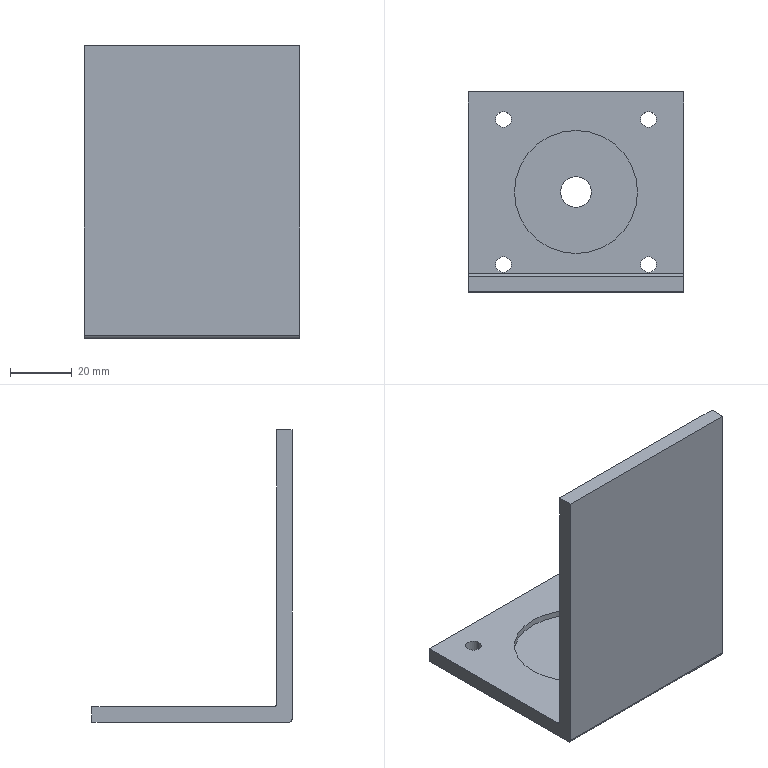Part | SolidWorks | features ICE 4, Fillet 2, Extrusion 1 | 1 solid | 23 faces | box 70 x 65 x 95 mm | volume 51093 mm3 | cylinder 14 | plane 9 | commonest cylinder face diameters 5.1 x8 2 x2 10 x2 40 x2
STEP:
#1=CARTESIAN_POINT('',(-5.,0.,0.));
#2=VERTEX_POINT('',#1);
#3=CARTESIAN_POINT('',(5.,0.,0.));
#4=VERTEX_POINT('',#3);
#5=CARTESIAN_POINT('',(0.,0.,0.));
#6=DIRECTION('',(0.,0.,1.));
#7=DIRECTION('',(1.,0.,0.));
#8=AXIS2_PLACEMENT_3D('',#5,#6,#7);
#9=CIRCLE('',#8,5.);
#10=EDGE_CURVE('',#2,#4,#9,.T.);
#11=ORIENTED_EDGE('',*,*,#10,.F.);
#12=CARTESIAN_POINT('',(-5.,0.,3.));
#13=VERTEX_POINT('',#12);
#14=CARTESIAN_POINT('',(-5.,0.,0.));
#15=DIRECTION('',(0.,0.,1.));
#16=VECTOR('',#15,1000.);
#17=LINE('',#14,#16);
#18=EDGE_CURVE('',#2,#13,#17,.T.);
#19=ORIENTED_EDGE('',*,*,#18,.T.);
#20=CARTESIAN_POINT('',(5.,0.,3.));
#21=VERTEX_POINT('',#20);
#22=CARTESIAN_POINT('',(0.,0.,3.));
#23=DIRECTION('',(0.,0.,1.));
#24=DIRECTION('',(1.,0.,0.));
#25=AXIS2_PLACEMENT_3D('',#22,#23,#24);
#26=CIRCLE('',#25,5.);
#27=EDGE_CURVE('',#13,#21,#26,.T.);
#28=ORIENTED_EDGE('',*,*,#27,.T.);
#29=CARTESIAN_POINT('',(5.,0.,0.));
#30=DIRECTION('',(0.,0.,1.));
#31=VECTOR('',#30,1000.);
#32=LINE('',#29,#31);
#33=EDGE_CURVE('',#4,#21,#32,.T.);
#34=ORIENTED_EDGE('',*,*,#33,.F.);
#35=EDGE_LOOP('',(#11,#19,#28,#34));
#36=FACE_OUTER_BOUND('',#35,.T.);
#37=CARTESIAN_POINT('',(0.,0.,0.));
#38=DIRECTION('',(0.,0.,1.));
#39=DIRECTION('',(1.,0.,0.));
#40=AXIS2_PLACEMENT_3D('',#37,#38,#39);
#41=CYLINDRICAL_SURFACE('',#40,5.);
#42=ADVANCED_FACE('',(#36),#41,.F.);
#43=CARTESIAN_POINT('',(-20.,0.,3.));
#44=VERTEX_POINT('',#43);
#45=CARTESIAN_POINT('',(20.,0.,3.));
#46=VERTEX_POINT('',#45);
#47=CARTESIAN_POINT('',(0.,0.,3.));
#48=DIRECTION('',(0.,0.,1.));
#49=DIRECTION('',(1.,0.,0.));
#50=AXIS2_PLACEMENT_3D('',#47,#48,#49);
#51=CIRCLE('',#50,20.);
#52=EDGE_CURVE('',#44,#46,#51,.T.);
#53=ORIENTED_EDGE('',*,*,#52,.F.);
#54=CARTESIAN_POINT('',(-20.,0.,5.));
#55=VERTEX_POINT('',#54);
#56=CARTESIAN_POINT('',(-20.,0.,3.));
#57=DIRECTION('',(0.,0.,1.));
#58=VECTOR('',#57,1000.);
#59=LINE('',#56,#58);
#60=EDGE_CURVE('',#44,#55,#59,.T.);
#61=ORIENTED_EDGE('',*,*,#60,.T.);
#62=CARTESIAN_POINT('',(20.,0.,5.));
#63=VERTEX_POINT('',#62);
#64=CARTESIAN_POINT('',(0.,0.,5.));
#65=DIRECTION('',(0.,0.,1.));
#66=DIRECTION('',(1.,0.,0.));
#67=AXIS2_PLACEMENT_3D('',#64,#65,#66);
#68=CIRCLE('',#67,20.);
#69=EDGE_CURVE('',#55,#63,#68,.T.);
#70=ORIENTED_EDGE('',*,*,#69,.T.);
#71=CARTESIAN_POINT('',(20.,0.,3.));
#72=DIRECTION('',(0.,0.,1.));
#73=VECTOR('',#72,1000.);
#74=LINE('',#71,#73);
#75=EDGE_CURVE('',#46,#63,#74,.T.);
#76=ORIENTED_EDGE('',*,*,#75,.F.);
#77=EDGE_LOOP('',(#53,#61,#70,#76));
#78=FACE_OUTER_BOUND('',#77,.T.);
#79=CARTESIAN_POINT('',(0.,0.,3.));
#80=DIRECTION('',(0.,0.,1.));
#81=DIRECTION('',(1.,0.,0.));
#82=AXIS2_PLACEMENT_3D('',#79,#80,#81);
#83=CYLINDRICAL_SURFACE('',#82,20.);
#84=ADVANCED_FACE('',(#78),#83,.F.);
#85=CARTESIAN_POINT('',(-26.12,-23.57,0.));
#86=VERTEX_POINT('',#85);
#87=CARTESIAN_POINT('',(-21.02,-23.57,0.));
#88=VERTEX_POINT('',#87);
#89=CARTESIAN_POINT('',(-23.57,-23.57,0.));
#90=DIRECTION('',(0.,0.,1.));
#91=DIRECTION('',(1.,0.,0.));
#92=AXIS2_PLACEMENT_3D('',#89,#90,#91);
#93=CIRCLE('',#92,2.55);
#94=EDGE_CURVE('',#86,#88,#93,.T.);
#95=ORIENTED_EDGE('',*,*,#94,.F.);
#96=CARTESIAN_POINT('',(-26.12,-23.57,5.));
#97=VERTEX_POINT('',#96);
#98=CARTESIAN_POINT('',(-26.12,-23.57,0.));
#99=DIRECTION('',(0.,0.,1.));
#100=VECTOR('',#99,1000.);
#101=LINE('',#98,#100);
#102=EDGE_CURVE('',#86,#97,#101,.T.);
#103=ORIENTED_EDGE('',*,*,#102,.T.);
#104=CARTESIAN_POINT('',(-21.02,-23.57,5.));
#105=VERTEX_POINT('',#104);
#106=CARTESIAN_POINT('',(-23.57,-23.57,5.));
#107=DIRECTION('',(0.,0.,1.));
#108=DIRECTION('',(1.,0.,0.));
#109=AXIS2_PLACEMENT_3D('',#106,#107,#108);
#110=CIRCLE('',#109,2.55);
#111=EDGE_CURVE('',#97,#105,#110,.T.);
#112=ORIENTED_EDGE('',*,*,#111,.T.);
#113=CARTESIAN_POINT('',(-21.02,-23.57,0.));
#114=DIRECTION('',(0.,0.,1.));
#115=VECTOR('',#114,1000.);
#116=LINE('',#113,#115);
#117=EDGE_CURVE('',#88,#105,#116,.T.);
#118=ORIENTED_EDGE('',*,*,#117,.F.);
#119=EDGE_LOOP('',(#95,#103,#112,#118));
#120=FACE_OUTER_BOUND('',#119,.T.);
#121=CARTESIAN_POINT('',(-23.57,-23.57,0.));
#122=DIRECTION('',(0.,0.,1.));
#123=DIRECTION('',(1.,0.,0.));
#124=AXIS2_PLACEMENT_3D('',#121,#122,#123);
#125=CYLINDRICAL_SURFACE('',#124,2.55);
#126=ADVANCED_FACE('',(#120),#125,.F.);
#127=CARTESIAN_POINT('',(21.02,-23.57,0.));
#128=VERTEX_POINT('',#127);
#129=CARTESIAN_POINT('',(26.12,-23.57,0.));
#130=VERTEX_POINT('',#129);
#131=CARTESIAN_POINT('',(23.57,-23.57,0.));
#132=DIRECTION('',(0.,0.,1.));
#133=DIRECTION('',(1.,0.,0.));
#134=AXIS2_PLACEMENT_3D('',#131,#132,#133);
#135=CIRCLE('',#134,2.55);
#136=EDGE_CURVE('',#128,#130,#135,.T.);
#137=ORIENTED_EDGE('',*,*,#136,.F.);
#138=CARTESIAN_POINT('',(21.02,-23.57,5.));
#139=VERTEX_POINT('',#138);
#140=CARTESIAN_POINT('',(21.02,-23.57,0.));
#141=DIRECTION('',(0.,0.,1.));
#142=VECTOR('',#141,1000.);
#143=LINE('',#140,#142);
#144=EDGE_CURVE('',#128,#139,#143,.T.);
#145=ORIENTED_EDGE('',*,*,#144,.T.);
#146=CARTESIAN_POINT('',(26.12,-23.57,5.));
#147=VERTEX_POINT('',#146);
#148=CARTESIAN_POINT('',(23.57,-23.57,5.));
#149=DIRECTION('',(0.,0.,1.));
#150=DIRECTION('',(1.,0.,0.));
#151=AXIS2_PLACEMENT_3D('',#148,#149,#150);
#152=CIRCLE('',#151,2.55);
#153=EDGE_CURVE('',#139,#147,#152,.T.);
#154=ORIENTED_EDGE('',*,*,#153,.T.);
#155=CARTESIAN_POINT('',(26.12,-23.57,0.));
#156=DIRECTION('',(0.,0.,1.));
#157=VECTOR('',#156,1000.);
#158=LINE('',#155,#157);
#159=EDGE_CURVE('',#130,#147,#158,.T.);
#160=ORIENTED_EDGE('',*,*,#159,.F.);
#161=EDGE_LOOP('',(#137,#145,#154,#160));
#162=FACE_OUTER_BOUND('',#161,.T.);
#163=CARTESIAN_POINT('',(23.57,-23.57,0.));
#164=DIRECTION('',(0.,0.,1.));
#165=DIRECTION('',(1.,0.,0.));
#166=AXIS2_PLACEMENT_3D('',#163,#164,#165);
#167=CYLINDRICAL_SURFACE('',#166,2.55);
#168=ADVANCED_FACE('',(#162),#167,.F.);
#169=CARTESIAN_POINT('',(21.02,23.57,0.));
#170=VERTEX_POINT('',#169);
#171=CARTESIAN_POINT('',(26.12,23.57,0.));
#172=VERTEX_POINT('',#171);
#173=CARTESIAN_POINT('',(23.57,23.57,0.));
#174=DIRECTION('',(0.,0.,1.));
#175=DIRECTION('',(1.,0.,0.));
#176=AXIS2_PLACEMENT_3D('',#173,#174,#175);
#177=CIRCLE('',#176,2.55);
#178=EDGE_CURVE('',#170,#172,#177,.T.);
#179=ORIENTED_EDGE('',*,*,#178,.F.);
#180=CARTESIAN_POINT('',(21.02,23.57,5.));
#181=VERTEX_POINT('',#180);
#182=CARTESIAN_POINT('',(21.02,23.57,0.));
#183=DIRECTION('',(0.,0.,1.));
#184=VECTOR('',#183,1000.);
#185=LINE('',#182,#184);
#186=EDGE_CURVE('',#170,#181,#185,.T.);
#187=ORIENTED_EDGE('',*,*,#186,.T.);
#188=CARTESIAN_POINT('',(26.12,23.57,5.));
#189=VERTEX_POINT('',#188);
#190=CARTESIAN_POINT('',(23.57,23.57,5.));
#191=DIRECTION('',(0.,0.,1.));
#192=DIRECTION('',(1.,0.,0.));
#193=AXIS2_PLACEMENT_3D('',#190,#191,#192);
#194=CIRCLE('',#193,2.55);
#195=EDGE_CURVE('',#181,#189,#194,.T.);
#196=ORIENTED_EDGE('',*,*,#195,.T.);
#197=CARTESIAN_POINT('',(26.12,23.57,0.));
#198=DIRECTION('',(0.,0.,1.));
#199=VECTOR('',#198,1000.);
#200=LINE('',#197,#199);
#201=EDGE_CURVE('',#172,#189,#200,.T.);
#202=ORIENTED_EDGE('',*,*,#201,.F.);
#203=EDGE_LOOP('',(#179,#187,#196,#202));
#204=FACE_OUTER_BOUND('',#203,.T.);
#205=CARTESIAN_POINT('',(23.57,23.57,0.));
#206=DIRECTION('',(0.,0.,1.));
#207=DIRECTION('',(1.,0.,0.));
#208=AXIS2_PLACEMENT_3D('',#205,#206,#207);
#209=CYLINDRICAL_SURFACE('',#208,2.55);
#210=ADVANCED_FACE('',(#204),#209,.F.);
#211=CARTESIAN_POINT('',(-26.12,23.57,0.));
#212=VERTEX_POINT('',#211);
#213=CARTESIAN_POINT('',(-21.02,23.57,0.));
#214=VERTEX_POINT('',#213);
#215=CARTESIAN_POINT('',(-23.57,23.57,0.));
#216=DIRECTION('',(0.,0.,1.));
#217=DIRECTION('',(1.,0.,0.));
#218=AXIS2_PLACEMENT_3D('',#215,#216,#217);
#219=CIRCLE('',#218,2.55);
#220=EDGE_CURVE('',#212,#214,#219,.T.);
#221=ORIENTED_EDGE('',*,*,#220,.F.);
#222=CARTESIAN_POINT('',(-26.12,23.57,5.));
#223=VERTEX_POINT('',#222);
#224=CARTESIAN_POINT('',(-26.12,23.57,0.));
#225=DIRECTION('',(0.,0.,1.));
#226=VECTOR('',#225,1000.);
#227=LINE('',#224,#226);
#228=EDGE_CURVE('',#212,#223,#227,.T.);
#229=ORIENTED_EDGE('',*,*,#228,.T.);
#230=CARTESIAN_POINT('',(-21.02,23.57,5.));
#231=VERTEX_POINT('',#230);
#232=CARTESIAN_POINT('',(-23.57,23.57,5.));
#233=DIRECTION('',(0.,0.,1.));
#234=DIRECTION('',(1.,0.,0.));
#235=AXIS2_PLACEMENT_3D('',#232,#233,#234);
#236=CIRCLE('',#235,2.55);
#237=EDGE_CURVE('',#223,#231,#236,.T.);
#238=ORIENTED_EDGE('',*,*,#237,.T.);
#239=CARTESIAN_POINT('',(-21.02,23.57,0.));
#240=DIRECTION('',(0.,0.,1.));
#241=VECTOR('',#240,1000.);
#242=LINE('',#239,#241);
#243=EDGE_CURVE('',#214,#231,#242,.T.);
#244=ORIENTED_EDGE('',*,*,#243,.F.);
#245=EDGE_LOOP('',(#221,#229,#238,#244));
#246=FACE_OUTER_BOUND('',#245,.T.);
#247=CARTESIAN_POINT('',(-23.57,23.57,0.));
#248=DIRECTION('',(0.,0.,1.));
#249=DIRECTION('',(1.,0.,0.));
#250=AXIS2_PLACEMENT_3D('',#247,#248,#249);
#251=CYLINDRICAL_SURFACE('',#250,2.55);
#252=ADVANCED_FACE('',(#246),#251,.F.);
#253=CARTESIAN_POINT('',(-35.,32.5,0.));
#254=VERTEX_POINT('',#253);
#255=CARTESIAN_POINT('',(35.,32.5,0.));
#256=VERTEX_POINT('',#255);
#257=CARTESIAN_POINT('',(-35.,32.5,0.));
#258=DIRECTION('',(1.,0.,0.));
#259=VECTOR('',#258,1000.);
#260=LINE('',#257,#259);
#261=EDGE_CURVE('',#254,#256,#260,.T.);
#262=ORIENTED_EDGE('',*,*,#261,.F.);
#263=CARTESIAN_POINT('',(-35.,32.5,5.));
#264=VERTEX_POINT('',#263);
#265=CARTESIAN_POINT('',(-35.,32.5,5.));
#266=DIRECTION('',(0.,0.,-1.));
#267=VECTOR('',#266,1000.);
#268=LINE('',#265,#267);
#269=EDGE_CURVE('',#264,#254,#268,.T.);
#270=ORIENTED_EDGE('',*,*,#269,.F.);
#271=CARTESIAN_POINT('',(35.,32.5,5.));
#272=VERTEX_POINT('',#271);
#273=CARTESIAN_POINT('',(-35.,32.5,5.));
#274=DIRECTION('',(1.,0.,0.));
#275=VECTOR('',#274,1000.);
#276=LINE('',#273,#275);
#277=EDGE_CURVE('',#264,#272,#276,.T.);
#278=ORIENTED_EDGE('',*,*,#277,.T.);
#279=CARTESIAN_POINT('',(35.,32.5,5.));
#280=DIRECTION('',(0.,0.,-1.));
#281=VECTOR('',#280,1000.);
#282=LINE('',#279,#281);
#283=EDGE_CURVE('',#272,#256,#282,.T.);
#284=ORIENTED_EDGE('',*,*,#283,.T.);
#285=EDGE_LOOP('',(#262,#270,#278,#284));
#286=FACE_OUTER_BOUND('',#285,.T.);
#287=CARTESIAN_POINT('',(-35.,32.5,5.));
#288=DIRECTION('',(0.,1.,0.));
#289=DIRECTION('',(0.,0.,1.));
#290=AXIS2_PLACEMENT_3D('',#287,#288,#289);
#291=PLANE('',#290);
#292=ADVANCED_FACE('',(#286),#291,.T.);
#293=CARTESIAN_POINT('',(-35.,-31.5,0.));
#294=VERTEX_POINT('',#293);
#295=CARTESIAN_POINT('',(-35.,-32.5,0.));
#296=DIRECTION('',(0.,1.,0.));
#297=VECTOR('',#296,1000.);
#298=LINE('',#295,#297);
#299=EDGE_CURVE('',#294,#254,#298,.T.);
#300=ORIENTED_EDGE('',*,*,#299,.F.);
#301=CARTESIAN_POINT('',(-35.,-32.5,1.));
#302=VERTEX_POINT('',#301);
#303=CARTESIAN_POINT('',(-35.,-31.5,1.));
#304=DIRECTION('',(-1.,0.,0.));
#305=DIRECTION('',(0.,0.,1.));
#306=AXIS2_PLACEMENT_3D('',#303,#304,#305);
#307=CIRCLE('',#306,1.);
#308=EDGE_CURVE('',#294,#302,#307,.T.);
#309=ORIENTED_EDGE('',*,*,#308,.T.);
#310=CARTESIAN_POINT('',(-35.,-32.5,95.));
#311=VERTEX_POINT('',#310);
#312=CARTESIAN_POINT('',(-35.,-32.5,5.));
#313=DIRECTION('',(0.,0.,-1.));
#314=VECTOR('',#313,1000.);
#315=LINE('',#312,#314);
#316=EDGE_CURVE('',#311,#302,#315,.T.);
#317=ORIENTED_EDGE('',*,*,#316,.F.);
#318=CARTESIAN_POINT('',(-35.,-27.5,95.));
#319=VERTEX_POINT('',#318);
#320=CARTESIAN_POINT('',(-35.,-32.5,95.));
#321=DIRECTION('',(0.,-1.,0.));
#322=VECTOR('',#321,1000.);
#323=LINE('',#320,#322);
#324=EDGE_CURVE('',#319,#311,#323,.T.);
#325=ORIENTED_EDGE('',*,*,#324,.F.);
#326=CARTESIAN_POINT('',(-35.,-27.5,6.));
#327=VERTEX_POINT('',#326);
#328=CARTESIAN_POINT('',(-35.,-27.5,95.));
#329=DIRECTION('',(0.,0.,-1.));
#330=VECTOR('',#329,1000.);
#331=LINE('',#328,#330);
#332=EDGE_CURVE('',#319,#327,#331,.T.);
#333=ORIENTED_EDGE('',*,*,#332,.T.);
#334=CARTESIAN_POINT('',(-35.,-26.5,5.));
#335=VERTEX_POINT('',#334);
#336=CARTESIAN_POINT('',(-35.,-26.5,6.));
#337=DIRECTION('',(1.,0.,0.));
#338=DIRECTION('',(0.,0.,1.));
#339=AXIS2_PLACEMENT_3D('',#336,#337,#338);
#340=CIRCLE('',#339,1.);
#341=EDGE_CURVE('',#327,#335,#340,.T.);
#342=ORIENTED_EDGE('',*,*,#341,.T.);
#343=CARTESIAN_POINT('',(-35.,-32.5,5.));
#344=DIRECTION('',(0.,1.,0.));
#345=VECTOR('',#344,1000.);
#346=LINE('',#343,#345);
#347=EDGE_CURVE('',#335,#264,#346,.T.);
#348=ORIENTED_EDGE('',*,*,#347,.T.);
#349=ORIENTED_EDGE('',*,*,#269,.T.);
#350=EDGE_LOOP('',(#300,#309,#317,#325,#333,#342,#348,#349));
#351=FACE_OUTER_BOUND('',#350,.T.);
#352=CARTESIAN_POINT('',(-35.,-32.5,5.));
#353=DIRECTION('',(-1.,0.,0.));
#354=DIRECTION('',(0.,0.,1.));
#355=AXIS2_PLACEMENT_3D('',#352,#353,#354);
#356=PLANE('',#355);
#357=ADVANCED_FACE('',(#351),#356,.T.);
#358=ORIENTED_EDGE('',*,*,#316,.T.);
#359=CARTESIAN_POINT('',(35.,-32.5,1.));
#360=VERTEX_POINT('',#359);
#361=CARTESIAN_POINT('',(-35.,-32.5,1.));
#362=DIRECTION('',(1.,0.,0.));
#363=VECTOR('',#362,1000.);
#364=LINE('',#361,#363);
#365=EDGE_CURVE('',#302,#360,#364,.T.);
#366=ORIENTED_EDGE('',*,*,#365,.T.);
#367=CARTESIAN_POINT('',(35.,-32.5,95.));
#368=VERTEX_POINT('',#367);
#369=CARTESIAN_POINT('',(35.,-32.5,5.));
#370=DIRECTION('',(0.,0.,-1.));
#371=VECTOR('',#370,1000.);
#372=LINE('',#369,#371);
#373=EDGE_CURVE('',#368,#360,#372,.T.);
#374=ORIENTED_EDGE('',*,*,#373,.F.);
#375=CARTESIAN_POINT('',(-35.,-32.5,95.));
#376=DIRECTION('',(1.,0.,0.));
#377=VECTOR('',#376,1000.);
#378=LINE('',#375,#377);
#379=EDGE_CURVE('',#311,#368,#378,.T.);
#380=ORIENTED_EDGE('',*,*,#379,.F.);
#381=EDGE_LOOP('',(#358,#366,#374,#380));
#382=FACE_OUTER_BOUND('',#381,.T.);
#383=CARTESIAN_POINT('',(-35.,-32.5,5.));
#384=DIRECTION('',(0.,1.,0.));
#385=DIRECTION('',(0.,0.,1.));
#386=AXIS2_PLACEMENT_3D('',#383,#384,#385);
#387=PLANE('',#386);
#388=ADVANCED_FACE('',(#382),#387,.F.);
#389=ORIENTED_EDGE('',*,*,#373,.T.);
#390=CARTESIAN_POINT('',(35.,-31.5,0.));
#391=VERTEX_POINT('',#390);
#392=CARTESIAN_POINT('',(35.,-31.5,1.));
#393=DIRECTION('',(1.,0.,0.));
#394=DIRECTION('',(0.,0.,1.));
#395=AXIS2_PLACEMENT_3D('',#392,#393,#394);
#396=CIRCLE('',#395,1.);
#397=EDGE_CURVE('',#360,#391,#396,.T.);
#398=ORIENTED_EDGE('',*,*,#397,.T.);
#399=CARTESIAN_POINT('',(35.,-32.5,0.));
#400=DIRECTION('',(0.,1.,0.));
#401=VECTOR('',#400,1000.);
#402=LINE('',#399,#401);
#403=EDGE_CURVE('',#391,#256,#402,.T.);
#404=ORIENTED_EDGE('',*,*,#403,.T.);
#405=ORIENTED_EDGE('',*,*,#283,.F.);
#406=CARTESIAN_POINT('',(35.,-26.5,5.));
#407=VERTEX_POINT('',#406);
#408=CARTESIAN_POINT('',(35.,-32.5,5.));
#409=DIRECTION('',(0.,1.,0.));
#410=VECTOR('',#409,1000.);
#411=LINE('',#408,#410);
#412=EDGE_CURVE('',#407,#272,#411,.T.);
#413=ORIENTED_EDGE('',*,*,#412,.F.);
#414=CARTESIAN_POINT('',(35.,-27.5,6.));
#415=VERTEX_POINT('',#414);
#416=CARTESIAN_POINT('',(35.,-26.5,6.));
#417=DIRECTION('',(-1.,0.,0.));
#418=DIRECTION('',(0.,0.,1.));
#419=AXIS2_PLACEMENT_3D('',#416,#417,#418);
#420=CIRCLE('',#419,1.);
#421=EDGE_CURVE('',#407,#415,#420,.T.);
#422=ORIENTED_EDGE('',*,*,#421,.T.);
#423=CARTESIAN_POINT('',(35.,-27.5,95.));
#424=VERTEX_POINT('',#423);
#425=CARTESIAN_POINT('',(35.,-27.5,95.));
#426=DIRECTION('',(0.,0.,-1.));
#427=VECTOR('',#426,1000.);
#428=LINE('',#425,#427);
#429=EDGE_CURVE('',#424,#415,#428,.T.);
#430=ORIENTED_EDGE('',*,*,#429,.F.);
#431=CARTESIAN_POINT('',(35.,-32.5,95.));
#432=DIRECTION('',(0.,1.,0.));
#433=VECTOR('',#432,1000.);
#434=LINE('',#431,#433);
#435=EDGE_CURVE('',#368,#424,#434,.T.);
#436=ORIENTED_EDGE('',*,*,#435,.F.);
#437=EDGE_LOOP('',(#389,#398,#404,#405,#413,#422,#430,#436));
#438=FACE_OUTER_BOUND('',#437,.T.);
#439=CARTESIAN_POINT('',(35.,-32.5,5.));
#440=DIRECTION('',(-1.,0.,0.));
#441=DIRECTION('',(0.,0.,1.));
#442=AXIS2_PLACEMENT_3D('',#439,#440,#441);
#443=PLANE('',#442);
#444=ADVANCED_FACE('',(#438),#443,.F.);
#445=CARTESIAN_POINT('',(0.,0.,5.));
#446=DIRECTION('',(0.,0.,1.));
#447=DIRECTION('',(1.,0.,0.));
#448=AXIS2_PLACEMENT_3D('',#445,#446,#447);
#449=CIRCLE('',#448,20.);
#450=EDGE_CURVE('',#63,#55,#449,.T.);
#451=ORIENTED_EDGE('',*,*,#450,.F.);
#452=ORIENTED_EDGE('',*,*,#69,.F.);
#453=EDGE_LOOP('',(#451,#452));
#454=FACE_BOUND('',#453,.T.);
#455=ORIENTED_EDGE('',*,*,#347,.F.);
#456=CARTESIAN_POINT('',(0.,-26.5,5.));
#457=DIRECTION('',(1.,0.,0.));
#458=VECTOR('',#457,1000.);
#459=LINE('',#456,#458);
#460=EDGE_CURVE('',#335,#407,#459,.T.);
#461=ORIENTED_EDGE('',*,*,#460,.T.);
#462=ORIENTED_EDGE('',*,*,#412,.T.);
#463=ORIENTED_EDGE('',*,*,#277,.F.);
#464=EDGE_LOOP('',(#455,#461,#462,#463));
#465=FACE_OUTER_BOUND('',#464,.T.);
#466=CARTESIAN_POINT('',(-23.57,-23.57,5.));
#467=DIRECTION('',(0.,0.,1.));
#468=DIRECTION('',(1.,0.,0.));
#469=AXIS2_PLACEMENT_3D('',#466,#467,#468);
#470=CIRCLE('',#469,2.55);
#471=EDGE_CURVE('',#105,#97,#470,.T.);
#472=ORIENTED_EDGE('',*,*,#471,.F.);
#473=ORIENTED_EDGE('',*,*,#111,.F.);
#474=EDGE_LOOP('',(#472,#473));
#475=FACE_BOUND('',#474,.T.);
#476=CARTESIAN_POINT('',(23.57,-23.57,5.));
#477=DIRECTION('',(0.,0.,1.));
#478=DIRECTION('',(1.,0.,0.));
#479=AXIS2_PLACEMENT_3D('',#476,#477,#478);
#480=CIRCLE('',#479,2.55);
#481=EDGE_CURVE('',#147,#139,#480,.T.);
#482=ORIENTED_EDGE('',*,*,#481,.F.);
#483=ORIENTED_EDGE('',*,*,#153,.F.);
#484=EDGE_LOOP('',(#482,#483));
#485=FACE_BOUND('',#484,.T.);
#486=CARTESIAN_POINT('',(23.57,23.57,5.));
#487=DIRECTION('',(0.,0.,1.));
#488=DIRECTION('',(1.,0.,0.));
#489=AXIS2_PLACEMENT_3D('',#486,#487,#488);
#490=CIRCLE('',#489,2.55);
#491=EDGE_CURVE('',#189,#181,#490,.T.);
#492=ORIENTED_EDGE('',*,*,#491,.F.);
#493=ORIENTED_EDGE('',*,*,#195,.F.);
#494=EDGE_LOOP('',(#492,#493));
#495=FACE_BOUND('',#494,.T.);
#496=CARTESIAN_POINT('',(-23.57,23.57,5.));
#497=DIRECTION('',(0.,0.,1.));
#498=DIRECTION('',(1.,0.,0.));
#499=AXIS2_PLACEMENT_3D('',#496,#497,#498);
#500=CIRCLE('',#499,2.55);
#501=EDGE_CURVE('',#231,#223,#500,.T.);
#502=ORIENTED_EDGE('',*,*,#501,.F.);
#503=ORIENTED_EDGE('',*,*,#237,.F.);
#504=EDGE_LOOP('',(#502,#503));
#505=FACE_BOUND('',#504,.T.);
#506=CARTESIAN_POINT('',(0.,0.,5.));
#507=DIRECTION('',(0.,0.,1.));
#508=DIRECTION('',(1.,0.,0.));
#509=AXIS2_PLACEMENT_3D('',#506,#507,#508);
#510=PLANE('',#509);
#511=ADVANCED_FACE('',(#454,#465,#475,#485,#495,#505),#510,.T.);
#512=CARTESIAN_POINT('',(0.,0.,0.));
#513=DIRECTION('',(0.,0.,1.));
#514=DIRECTION('',(1.,0.,0.));
#515=AXIS2_PLACEMENT_3D('',#512,#513,#514);
#516=CIRCLE('',#515,5.);
#517=EDGE_CURVE('',#4,#2,#516,.T.);
#518=ORIENTED_EDGE('',*,*,#517,.T.);
#519=ORIENTED_EDGE('',*,*,#10,.T.);
#520=EDGE_LOOP('',(#518,#519));
#521=FACE_BOUND('',#520,.T.);
#522=CARTESIAN_POINT('',(-23.57,-23.57,0.));
#523=DIRECTION('',(0.,0.,1.));
#524=DIRECTION('',(1.,0.,0.));
#525=AXIS2_PLACEMENT_3D('',#522,#523,#524);
#526=CIRCLE('',#525,2.55);
#527=EDGE_CURVE('',#88,#86,#526,.T.);
#528=ORIENTED_EDGE('',*,*,#527,.T.);
#529=ORIENTED_EDGE('',*,*,#94,.T.);
#530=EDGE_LOOP('',(#528,#529));
#531=FACE_BOUND('',#530,.T.);
#532=CARTESIAN_POINT('',(23.57,-23.57,0.));
#533=DIRECTION('',(0.,0.,1.));
#534=DIRECTION('',(1.,0.,0.));
#535=AXIS2_PLACEMENT_3D('',#532,#533,#534);
#536=CIRCLE('',#535,2.55);
#537=EDGE_CURVE('',#130,#128,#536,.T.);
#538=ORIENTED_EDGE('',*,*,#537,.T.);
#539=ORIENTED_EDGE('',*,*,#136,.T.);
#540=EDGE_LOOP('',(#538,#539));
#541=FACE_BOUND('',#540,.T.);
#542=CARTESIAN_POINT('',(23.57,23.57,0.));
#543=DIRECTION('',(0.,0.,1.));
#544=DIRECTION('',(1.,0.,0.));
#545=AXIS2_PLACEMENT_3D('',#542,#543,#544);
#546=CIRCLE('',#545,2.55);
#547=EDGE_CURVE('',#172,#170,#546,.T.);
#548=ORIENTED_EDGE('',*,*,#547,.T.);
#549=ORIENTED_EDGE('',*,*,#178,.T.);
#550=EDGE_LOOP('',(#548,#549));
#551=FACE_BOUND('',#550,.T.);
#552=CARTESIAN_POINT('',(-23.57,23.57,0.));
#553=DIRECTION('',(0.,0.,1.));
#554=DIRECTION('',(1.,0.,0.));
#555=AXIS2_PLACEMENT_3D('',#552,#553,#554);
#556=CIRCLE('',#555,2.55);
#557=EDGE_CURVE('',#214,#212,#556,.T.);
#558=ORIENTED_EDGE('',*,*,#557,.T.);
#559=ORIENTED_EDGE('',*,*,#220,.T.);
#560=EDGE_LOOP('',(#558,#559));
#561=FACE_BOUND('',#560,.T.);
#562=ORIENTED_EDGE('',*,*,#403,.F.);
#563=CARTESIAN_POINT('',(0.,-31.5,0.));
#564=DIRECTION('',(-1.,0.,0.));
#565=VECTOR('',#564,1000.);
#566=LINE('',#563,#565);
#567=EDGE_CURVE('',#391,#294,#566,.T.);
#568=ORIENTED_EDGE('',*,*,#567,.T.);
#569=ORIENTED_EDGE('',*,*,#299,.T.);
#570=ORIENTED_EDGE('',*,*,#261,.T.);
#571=EDGE_LOOP('',(#562,#568,#569,#570));
#572=FACE_OUTER_BOUND('',#571,.T.);
#573=CARTESIAN_POINT('',(0.,0.,0.));
#574=DIRECTION('',(0.,0.,1.));
#575=DIRECTION('',(1.,0.,0.));
#576=AXIS2_PLACEMENT_3D('',#573,#574,#575);
#577=PLANE('',#576);
#578=ADVANCED_FACE('',(#521,#531,#541,#551,#561,#572),#577,.F.);
#579=ORIENTED_EDGE('',*,*,#228,.F.);
#580=ORIENTED_EDGE('',*,*,#557,.F.);
#581=ORIENTED_EDGE('',*,*,#243,.T.);
#582=ORIENTED_EDGE('',*,*,#501,.T.);
#583=EDGE_LOOP('',(#579,#580,#581,#582));
#584=FACE_OUTER_BOUND('',#583,.T.);
#585=CARTESIAN_POINT('',(-23.57,23.57,0.));
#586=DIRECTION('',(0.,0.,1.));
#587=DIRECTION('',(1.,0.,0.));
#588=AXIS2_PLACEMENT_3D('',#585,#586,#587);
#589=CYLINDRICAL_SURFACE('',#588,2.55);
#590=ADVANCED_FACE('',(#584),#589,.F.);
#591=ORIENTED_EDGE('',*,*,#186,.F.);
#592=ORIENTED_EDGE('',*,*,#547,.F.);
#593=ORIENTED_EDGE('',*,*,#201,.T.);
#594=ORIENTED_EDGE('',*,*,#491,.T.);
#595=EDGE_LOOP('',(#591,#592,#593,#594));
#596=FACE_OUTER_BOUND('',#595,.T.);
#597=CARTESIAN_POINT('',(23.57,23.57,0.));
#598=DIRECTION('',(0.,0.,1.));
#599=DIRECTION('',(1.,0.,0.));
#600=AXIS2_PLACEMENT_3D('',#597,#598,#599);
#601=CYLINDRICAL_SURFACE('',#600,2.55);
#602=ADVANCED_FACE('',(#596),#601,.F.);
#603=ORIENTED_EDGE('',*,*,#144,.F.);
#604=ORIENTED_EDGE('',*,*,#537,.F.);
#605=ORIENTED_EDGE('',*,*,#159,.T.);
#606=ORIENTED_EDGE('',*,*,#481,.T.);
#607=EDGE_LOOP('',(#603,#604,#605,#606));
#608=FACE_OUTER_BOUND('',#607,.T.);
#609=CARTESIAN_POINT('',(23.57,-23.57,0.));
#610=DIRECTION('',(0.,0.,1.));
#611=DIRECTION('',(1.,0.,0.));
#612=AXIS2_PLACEMENT_3D('',#609,#610,#611);
#613=CYLINDRICAL_SURFACE('',#612,2.55);
#614=ADVANCED_FACE('',(#608),#613,.F.);
#615=ORIENTED_EDGE('',*,*,#102,.F.);
#616=ORIENTED_EDGE('',*,*,#527,.F.);
#617=ORIENTED_EDGE('',*,*,#117,.T.);
#618=ORIENTED_EDGE('',*,*,#471,.T.);
#619=EDGE_LOOP('',(#615,#616,#617,#618));
#620=FACE_OUTER_BOUND('',#619,.T.);
#621=CARTESIAN_POINT('',(-23.57,-23.57,0.));
#622=DIRECTION('',(0.,0.,1.));
#623=DIRECTION('',(1.,0.,0.));
#624=AXIS2_PLACEMENT_3D('',#621,#622,#623);
#625=CYLINDRICAL_SURFACE('',#624,2.55);
#626=ADVANCED_FACE('',(#620),#625,.F.);
#627=ORIENTED_EDGE('',*,*,#429,.T.);
#628=CARTESIAN_POINT('',(-35.,-27.5,6.));
#629=DIRECTION('',(-1.,0.,0.));
#630=VECTOR('',#629,1000.);
#631=LINE('',#628,#630);
#632=EDGE_CURVE('',#415,#327,#631,.T.);
#633=ORIENTED_EDGE('',*,*,#632,.T.);
#634=ORIENTED_EDGE('',*,*,#332,.F.);
#635=CARTESIAN_POINT('',(-35.,-27.5,95.));
#636=DIRECTION('',(-1.,0.,0.));
#637=VECTOR('',#636,1000.);
#638=LINE('',#635,#637);
#639=EDGE_CURVE('',#424,#319,#638,.T.);
#640=ORIENTED_EDGE('',*,*,#639,.F.);
#641=EDGE_LOOP('',(#627,#633,#634,#640));
#642=FACE_OUTER_BOUND('',#641,.T.);
#643=CARTESIAN_POINT('',(-35.,-27.5,95.));
#644=DIRECTION('',(0.,-1.,0.));
#645=DIRECTION('',(0.,0.,-1.));
#646=AXIS2_PLACEMENT_3D('',#643,#644,#645);
#647=PLANE('',#646);
#648=ADVANCED_FACE('',(#642),#647,.F.);
#649=ORIENTED_EDGE('',*,*,#324,.T.);
#650=ORIENTED_EDGE('',*,*,#379,.T.);
#651=ORIENTED_EDGE('',*,*,#435,.T.);
#652=ORIENTED_EDGE('',*,*,#639,.T.);
#653=EDGE_LOOP('',(#649,#650,#651,#652));
#654=FACE_OUTER_BOUND('',#653,.T.);
#655=CARTESIAN_POINT('',(0.,0.,95.));
#656=DIRECTION('',(0.,0.,-1.));
#657=DIRECTION('',(-1.,0.,0.));
#658=AXIS2_PLACEMENT_3D('',#655,#656,#657);
#659=PLANE('',#658);
#660=ADVANCED_FACE('',(#654),#659,.F.);
#661=ORIENTED_EDGE('',*,*,#421,.F.);
#662=ORIENTED_EDGE('',*,*,#460,.F.);
#663=ORIENTED_EDGE('',*,*,#341,.F.);
#664=ORIENTED_EDGE('',*,*,#632,.F.);
#665=EDGE_LOOP('',(#661,#662,#663,#664));
#666=FACE_OUTER_BOUND('',#665,.T.);
#667=CARTESIAN_POINT('',(-35.,-26.5,6.));
#668=DIRECTION('',(-1.,0.,0.));
#669=DIRECTION('',(0.,0.,1.));
#670=AXIS2_PLACEMENT_3D('',#667,#668,#669);
#671=CYLINDRICAL_SURFACE('',#670,1.);
#672=ADVANCED_FACE('',(#666),#671,.F.);
#673=ORIENTED_EDGE('',*,*,#308,.F.);
#674=ORIENTED_EDGE('',*,*,#567,.F.);
#675=ORIENTED_EDGE('',*,*,#397,.F.);
#676=ORIENTED_EDGE('',*,*,#365,.F.);
#677=EDGE_LOOP('',(#673,#674,#675,#676));
#678=FACE_OUTER_BOUND('',#677,.T.);
#679=CARTESIAN_POINT('',(-35.,-31.5,1.));
#680=DIRECTION('',(1.,0.,0.));
#681=DIRECTION('',(0.,0.,-1.));
#682=AXIS2_PLACEMENT_3D('',#679,#680,#681);
#683=CYLINDRICAL_SURFACE('',#682,1.);
#684=ADVANCED_FACE('',(#678),#683,.T.);
#685=ORIENTED_EDGE('',*,*,#60,.F.);
#686=CARTESIAN_POINT('',(0.,0.,3.));
#687=DIRECTION('',(0.,0.,1.));
#688=DIRECTION('',(1.,0.,0.));
#689=AXIS2_PLACEMENT_3D('',#686,#687,#688);
#690=CIRCLE('',#689,20.);
#691=EDGE_CURVE('',#46,#44,#690,.T.);
#692=ORIENTED_EDGE('',*,*,#691,.F.);
#693=ORIENTED_EDGE('',*,*,#75,.T.);
#694=ORIENTED_EDGE('',*,*,#450,.T.);
#695=EDGE_LOOP('',(#685,#692,#693,#694));
#696=FACE_OUTER_BOUND('',#695,.T.);
#697=CARTESIAN_POINT('',(0.,0.,3.));
#698=DIRECTION('',(0.,0.,1.));
#699=DIRECTION('',(1.,0.,0.));
#700=AXIS2_PLACEMENT_3D('',#697,#698,#699);
#701=CYLINDRICAL_SURFACE('',#700,20.);
#702=ADVANCED_FACE('',(#696),#701,.F.);
#703=CARTESIAN_POINT('',(0.,0.,3.));
#704=DIRECTION('',(0.,0.,1.));
#705=DIRECTION('',(1.,0.,0.));
#706=AXIS2_PLACEMENT_3D('',#703,#704,#705);
#707=CIRCLE('',#706,5.);
#708=EDGE_CURVE('',#21,#13,#707,.T.);
#709=ORIENTED_EDGE('',*,*,#708,.F.);
#710=ORIENTED_EDGE('',*,*,#27,.F.);
#711=EDGE_LOOP('',(#709,#710));
#712=FACE_BOUND('',#711,.T.);
#713=ORIENTED_EDGE('',*,*,#691,.T.);
#714=ORIENTED_EDGE('',*,*,#52,.T.);
#715=EDGE_LOOP('',(#713,#714));
#716=FACE_OUTER_BOUND('',#715,.T.);
#717=CARTESIAN_POINT('',(0.,0.,3.));
#718=DIRECTION('',(0.,0.,1.));
#719=DIRECTION('',(1.,0.,0.));
#720=AXIS2_PLACEMENT_3D('',#717,#718,#719);
#721=PLANE('',#720);
#722=ADVANCED_FACE('',(#712,#716),#721,.T.);
#723=ORIENTED_EDGE('',*,*,#18,.F.);
#724=ORIENTED_EDGE('',*,*,#517,.F.);
#725=ORIENTED_EDGE('',*,*,#33,.T.);
#726=ORIENTED_EDGE('',*,*,#708,.T.);
#727=EDGE_LOOP('',(#723,#724,#725,#726));
#728=FACE_OUTER_BOUND('',#727,.T.);
#729=CARTESIAN_POINT('',(0.,0.,0.));
#730=DIRECTION('',(0.,0.,1.));
#731=DIRECTION('',(1.,0.,0.));
#732=AXIS2_PLACEMENT_3D('',#729,#730,#731);
#733=CYLINDRICAL_SURFACE('',#732,5.);
#734=ADVANCED_FACE('',(#728),#733,.F.);
#735=CLOSED_SHELL('',(#42,#84,#126,#168,#210,#252,#292,#357,#388,#444,#511,#578,#590,#602,#614,#626,#648,#660,#672,#684,#702,#722,#734));
#736=MANIFOLD_SOLID_BREP('',#735);
#737=CARTESIAN_POINT('',(0.,0.,0.));
#738=DIRECTION('',(0.,0.,1.));
#739=DIRECTION('',(1.,0.,0.));
#740=AXIS2_PLACEMENT_3D('',#737,#738,#739);
#741=(LENGTH_UNIT()NAMED_UNIT(*)SI_UNIT(.MILLI.,.METRE.));
#742=UNCERTAINTY_MEASURE_WITH_UNIT(LENGTH_MEASURE(0.00001),#741,'','');
#743=(NAMED_UNIT(*)PLANE_ANGLE_UNIT()SI_UNIT($,.RADIAN.));
#744=(NAMED_UNIT(*)SI_UNIT($,.STERADIAN.)SOLID_ANGLE_UNIT());
#745=(GEOMETRIC_REPRESENTATION_CONTEXT(3)GLOBAL_UNCERTAINTY_ASSIGNED_CONTEXT((#742))GLOBAL_UNIT_ASSIGNED_CONTEXT((#741,#743,#744))REPRESENTATION_CONTEXT('',''));
#746=ADVANCED_BREP_SHAPE_REPRESENTATION('',(#736,#740),#745);